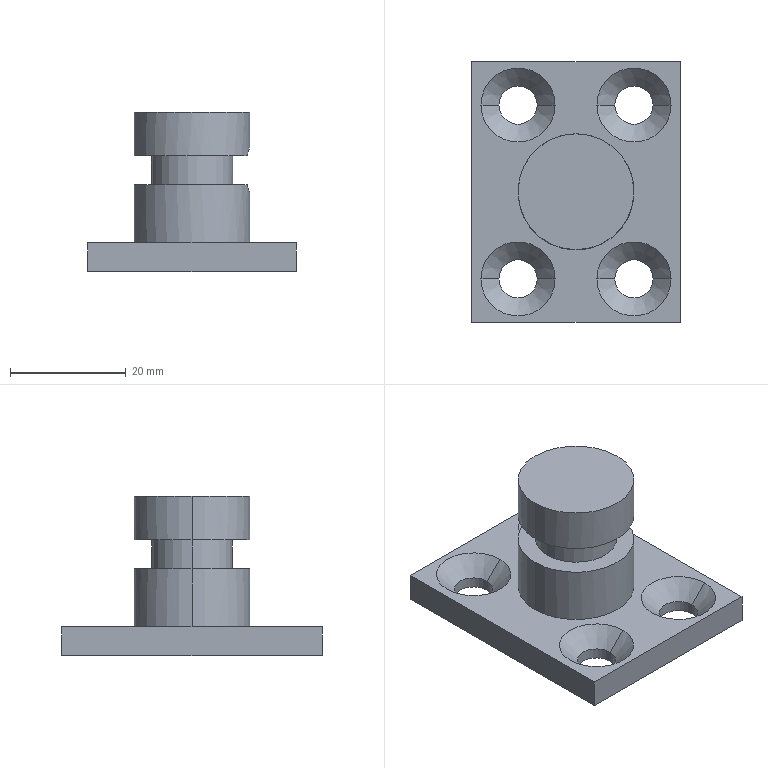Part | STEP file | Traction holder seat QY-1-39 | 2 solids | 35 faces | box 36 x 45 x 27.5 mm | volume 13120 mm3 | cylinder 17 | plane 10 | cone 8 | commonest cylinder face diameters 6.6 x8 20 x4 8 x3 14 x2